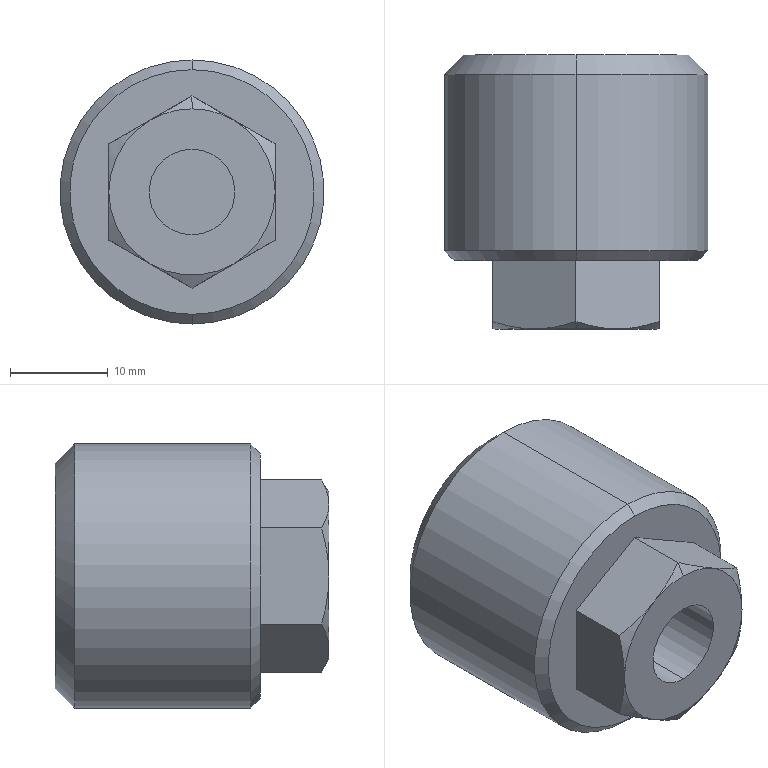Part | 1 solid | 29 faces | box 27 x 28 x 27 mm | volume 12379 mm3 | cone 11 | plane 10 | cylinder 6 | sphere 2 | commonest cylinder face diameters 8.75 x2 10 x2 27 x2
STEP:
#1=CARTESIAN_POINT('',(0.,18.,-5.));
#2=VERTEX_POINT('',#1);
#3=CARTESIAN_POINT('',(0.,18.,5.));
#4=VERTEX_POINT('',#3);
#5=CARTESIAN_POINT('',(0.,18.,0.));
#6=DIRECTION('',(0.,1.,0.));
#7=DIRECTION('',(0.,0.,-1.));
#8=AXIS2_PLACEMENT_3D('',#5,#6,#7);
#9=CIRCLE('',#8,5.);
#10=EDGE_CURVE('',#2,#4,#9,.T.);
#11=ORIENTED_EDGE('',*,*,#10,.T.);
#12=CARTESIAN_POINT('',(0.,13.,0.));
#13=VERTEX_POINT('',#12);
#14=CARTESIAN_POINT('',(0.,18.,0.));
#15=DIRECTION('',(1.,0.,0.));
#16=DIRECTION('',(0.,0.,-1.));
#17=AXIS2_PLACEMENT_3D('',#14,#15,#16);
#18=CIRCLE('',#17,5.);
#19=EDGE_CURVE('',#4,#13,#18,.T.);
#20=ORIENTED_EDGE('',*,*,#19,.T.);
#21=CARTESIAN_POINT('',(0.,18.,0.));
#22=DIRECTION('',(-1.,0.,0.));
#23=DIRECTION('',(0.,0.,1.));
#24=AXIS2_PLACEMENT_3D('',#21,#22,#23);
#25=CIRCLE('',#24,5.);
#26=EDGE_CURVE('',#2,#13,#25,.T.);
#27=ORIENTED_EDGE('',*,*,#26,.F.);
#28=EDGE_LOOP('',(#11,#20,#27));
#29=FACE_OUTER_BOUND('',#28,.T.);
#30=CARTESIAN_POINT('',(0.,18.,0.));
#31=DIRECTION('',(1.,0.,0.));
#32=DIRECTION('',(0.,0.,-1.));
#33=AXIS2_PLACEMENT_3D('',#30,#31,#32);
#34=SPHERICAL_SURFACE('',#33,5.);
#35=ADVANCED_FACE('',(#29),#34,.F.);
#36=CARTESIAN_POINT('',(0.,4.5,4.375));
#37=VERTEX_POINT('',#36);
#38=CARTESIAN_POINT('',(0.,4.5,-4.375));
#39=VERTEX_POINT('',#38);
#40=CARTESIAN_POINT('',(0.,4.5,0.));
#41=DIRECTION('',(0.,-1.,0.));
#42=DIRECTION('',(0.,0.,-1.));
#43=AXIS2_PLACEMENT_3D('',#40,#41,#42);
#44=CIRCLE('',#43,4.375);
#45=EDGE_CURVE('',#37,#39,#44,.T.);
#46=ORIENTED_EDGE('',*,*,#45,.F.);
#47=CARTESIAN_POINT('',(0.,-7.,4.375));
#48=VERTEX_POINT('',#47);
#49=CARTESIAN_POINT('',(0.,4.5,4.375));
#50=DIRECTION('',(0.,-1.,0.));
#51=VECTOR('',#50,1000.);
#52=LINE('',#49,#51);
#53=EDGE_CURVE('',#37,#48,#52,.T.);
#54=ORIENTED_EDGE('',*,*,#53,.T.);
#55=CARTESIAN_POINT('',(0.,-7.,-4.375));
#56=VERTEX_POINT('',#55);
#57=CARTESIAN_POINT('',(0.,-7.,0.));
#58=DIRECTION('',(0.,-1.,0.));
#59=DIRECTION('',(0.,0.,-1.));
#60=AXIS2_PLACEMENT_3D('',#57,#58,#59);
#61=CIRCLE('',#60,4.375);
#62=EDGE_CURVE('',#48,#56,#61,.T.);
#63=ORIENTED_EDGE('',*,*,#62,.T.);
#64=CARTESIAN_POINT('',(0.,4.5,-4.375));
#65=DIRECTION('',(0.,-1.,0.));
#66=VECTOR('',#65,1000.);
#67=LINE('',#64,#66);
#68=EDGE_CURVE('',#39,#56,#67,.T.);
#69=ORIENTED_EDGE('',*,*,#68,.F.);
#70=EDGE_LOOP('',(#46,#54,#63,#69));
#71=FACE_OUTER_BOUND('',#70,.T.);
#72=CARTESIAN_POINT('',(0.,4.5,0.));
#73=DIRECTION('',(0.,-1.,0.));
#74=DIRECTION('',(0.,0.,-1.));
#75=AXIS2_PLACEMENT_3D('',#72,#73,#74);
#76=CYLINDRICAL_SURFACE('',#75,4.375);
#77=ADVANCED_FACE('',(#71),#76,.F.);
#78=ORIENTED_EDGE('',*,*,#10,.F.);
#79=CARTESIAN_POINT('',(0.,21.,-5.));
#80=VERTEX_POINT('',#79);
#81=CARTESIAN_POINT('',(0.,18.,-5.));
#82=DIRECTION('',(0.,1.,0.));
#83=VECTOR('',#82,1000.);
#84=LINE('',#81,#83);
#85=EDGE_CURVE('',#2,#80,#84,.T.);
#86=ORIENTED_EDGE('',*,*,#85,.T.);
#87=CARTESIAN_POINT('',(0.,21.,5.));
#88=VERTEX_POINT('',#87);
#89=CARTESIAN_POINT('',(0.,21.,0.));
#90=DIRECTION('',(0.,-1.,0.));
#91=DIRECTION('',(0.,0.,-1.));
#92=AXIS2_PLACEMENT_3D('',#89,#90,#91);
#93=CIRCLE('',#92,5.);
#94=EDGE_CURVE('',#88,#80,#93,.T.);
#95=ORIENTED_EDGE('',*,*,#94,.F.);
#96=CARTESIAN_POINT('',(0.,18.,5.));
#97=DIRECTION('',(0.,1.,0.));
#98=VECTOR('',#97,1000.);
#99=LINE('',#96,#98);
#100=EDGE_CURVE('',#4,#88,#99,.T.);
#101=ORIENTED_EDGE('',*,*,#100,.F.);
#102=EDGE_LOOP('',(#78,#86,#95,#101));
#103=FACE_OUTER_BOUND('',#102,.T.);
#104=CARTESIAN_POINT('',(0.,18.,0.));
#105=DIRECTION('',(0.,1.,0.));
#106=DIRECTION('',(0.,0.,1.));
#107=AXIS2_PLACEMENT_3D('',#104,#105,#106);
#108=CYLINDRICAL_SURFACE('',#107,5.);
#109=ADVANCED_FACE('',(#103),#108,.F.);
#110=CARTESIAN_POINT('',(-4.25,-7.,7.361));
#111=VERTEX_POINT('',#110);
#112=CARTESIAN_POINT('',(0.,-7.,8.5));
#113=VERTEX_POINT('',#112);
#114=CARTESIAN_POINT('',(0.,-7.,0.));
#115=DIRECTION('',(0.,1.,0.));
#116=DIRECTION('',(0.,0.,1.));
#117=AXIS2_PLACEMENT_3D('',#114,#115,#116);
#118=CIRCLE('',#117,8.5);
#119=EDGE_CURVE('',#111,#113,#118,.T.);
#120=ORIENTED_EDGE('',*,*,#119,.T.);
#121=CARTESIAN_POINT('',(0.,-6.241,9.815));
#122=VERTEX_POINT('',#121);
#123=CARTESIAN_POINT('',(0.,8.034,34.54));
#124=DIRECTION('',(0.,0.5,0.866));
#125=VECTOR('',#124,1000.);
#126=LINE('',#123,#125);
#127=EDGE_CURVE('',#113,#122,#126,.T.);
#128=ORIENTED_EDGE('',*,*,#127,.T.);
#129=CARTESIAN_POINT('',(-4.25,-7.,7.361));
#130=CARTESIAN_POINT('',(-3.899,-7.,7.564));
#131=CARTESIAN_POINT('',(-3.367,-6.974,7.871));
#132=CARTESIAN_POINT('',(-2.737,-6.9,8.235));
#133=CARTESIAN_POINT('',(-2.42,-6.851,8.418));
#134=CARTESIAN_POINT('',(-2.26,-6.824,8.51));
#135=CARTESIAN_POINT('',(-2.18,-6.81,8.556));
#136=CARTESIAN_POINT('',(-2.146,-6.804,8.576));
#137=CARTESIAN_POINT('',(-2.123,-6.799,8.589));
#138=CARTESIAN_POINT('',(-2.111,-6.797,8.596));
#139=CARTESIAN_POINT('',(-1.437,-6.671,8.986));
#140=CARTESIAN_POINT('',(-0.7363,-6.486,9.39));
#141=CARTESIAN_POINT('',(0.,-6.241,9.815));
#142=B_SPLINE_CURVE_WITH_KNOTS('',3,(#129,#130,#131,#132,#133,#134,#135,#136,#137,#138,#139,#140,#141),.UNSPECIFIED.,.F.,.F.,(4,1,1,1,1,1,2,2,4),(0.,0.25,0.375,0.4375,0.4687,0.4844,0.4922,0.5,1.),.UNSPECIFIED.);
#143=EDGE_CURVE('',#111,#122,#142,.T.);
#144=ORIENTED_EDGE('',*,*,#143,.F.);
#145=EDGE_LOOP('',(#120,#128,#144));
#146=FACE_OUTER_BOUND('',#145,.T.);
#147=CARTESIAN_POINT('',(0.,8.034,0.));
#148=DIRECTION('',(0.,1.,0.));
#149=DIRECTION('',(0.,0.,1.));
#150=AXIS2_PLACEMENT_3D('',#147,#148,#149);
#151=CONICAL_SURFACE('',#150,34.54,1.047);
#152=ADVANCED_FACE('',(#146),#151,.T.);
#153=CARTESIAN_POINT('',(0.,0.,-12.5));
#154=VERTEX_POINT('',#153);
#155=CARTESIAN_POINT('',(0.,0.,12.5));
#156=VERTEX_POINT('',#155);
#157=CARTESIAN_POINT('',(0.,0.,0.));
#158=DIRECTION('',(0.,-1.,0.));
#159=DIRECTION('',(0.,0.,1.));
#160=AXIS2_PLACEMENT_3D('',#157,#158,#159);
#161=CIRCLE('',#160,12.5);
#162=EDGE_CURVE('',#154,#156,#161,.T.);
#163=ORIENTED_EDGE('',*,*,#162,.F.);
#164=CARTESIAN_POINT('',(0.,1.,-13.5));
#165=VERTEX_POINT('',#164);
#166=CARTESIAN_POINT('',(0.,1.,-13.5));
#167=DIRECTION('',(0.,0.7071,-0.7071));
#168=VECTOR('',#167,1000.);
#169=LINE('',#166,#168);
#170=EDGE_CURVE('',#154,#165,#169,.T.);
#171=ORIENTED_EDGE('',*,*,#170,.T.);
#172=CARTESIAN_POINT('',(0.,1.,13.5));
#173=VERTEX_POINT('',#172);
#174=CARTESIAN_POINT('',(0.,1.,0.));
#175=DIRECTION('',(0.,1.,0.));
#176=DIRECTION('',(0.,0.,1.));
#177=AXIS2_PLACEMENT_3D('',#174,#175,#176);
#178=CIRCLE('',#177,13.5);
#179=EDGE_CURVE('',#173,#165,#178,.T.);
#180=ORIENTED_EDGE('',*,*,#179,.F.);
#181=CARTESIAN_POINT('',(0.,1.,13.5));
#182=DIRECTION('',(0.,0.7071,0.7071));
#183=VECTOR('',#182,1000.);
#184=LINE('',#181,#183);
#185=EDGE_CURVE('',#156,#173,#184,.T.);
#186=ORIENTED_EDGE('',*,*,#185,.F.);
#187=EDGE_LOOP('',(#163,#171,#180,#186));
#188=FACE_OUTER_BOUND('',#187,.T.);
#189=CARTESIAN_POINT('',(0.,1.,0.));
#190=DIRECTION('',(0.,1.,0.));
#191=DIRECTION('',(0.,0.,1.));
#192=AXIS2_PLACEMENT_3D('',#189,#190,#191);
#193=CONICAL_SURFACE('',#192,13.5,0.7854);
#194=ADVANCED_FACE('',(#188),#193,.T.);
#195=CARTESIAN_POINT('',(0.,21.,11.5));
#196=VERTEX_POINT('',#195);
#197=CARTESIAN_POINT('',(0.,21.,-11.5));
#198=VERTEX_POINT('',#197);
#199=CARTESIAN_POINT('',(0.,21.,0.));
#200=DIRECTION('',(0.,1.,0.));
#201=DIRECTION('',(0.,0.,1.));
#202=AXIS2_PLACEMENT_3D('',#199,#200,#201);
#203=CIRCLE('',#202,11.5);
#204=EDGE_CURVE('',#196,#198,#203,.T.);
#205=ORIENTED_EDGE('',*,*,#204,.F.);
#206=CARTESIAN_POINT('',(0.,19.,13.5));
#207=VERTEX_POINT('',#206);
#208=CARTESIAN_POINT('',(0.,19.,13.5));
#209=DIRECTION('',(0.,-0.7071,0.7071));
#210=VECTOR('',#209,1000.);
#211=LINE('',#208,#210);
#212=EDGE_CURVE('',#196,#207,#211,.T.);
#213=ORIENTED_EDGE('',*,*,#212,.T.);
#214=CARTESIAN_POINT('',(0.,19.,-13.5));
#215=VERTEX_POINT('',#214);
#216=CARTESIAN_POINT('',(0.,19.,0.));
#217=DIRECTION('',(0.,1.,0.));
#218=DIRECTION('',(0.,0.,1.));
#219=AXIS2_PLACEMENT_3D('',#216,#217,#218);
#220=CIRCLE('',#219,13.5);
#221=EDGE_CURVE('',#207,#215,#220,.T.);
#222=ORIENTED_EDGE('',*,*,#221,.T.);
#223=CARTESIAN_POINT('',(0.,19.,-13.5));
#224=DIRECTION('',(0.,-0.7071,-0.7071));
#225=VECTOR('',#224,1000.);
#226=LINE('',#223,#225);
#227=EDGE_CURVE('',#198,#215,#226,.T.);
#228=ORIENTED_EDGE('',*,*,#227,.F.);
#229=EDGE_LOOP('',(#205,#213,#222,#228));
#230=FACE_OUTER_BOUND('',#229,.T.);
#231=CARTESIAN_POINT('',(0.,19.,0.));
#232=DIRECTION('',(0.,-1.,0.));
#233=DIRECTION('',(0.,0.,-1.));
#234=AXIS2_PLACEMENT_3D('',#231,#232,#233);
#235=CONICAL_SURFACE('',#234,13.5,0.7854);
#236=ADVANCED_FACE('',(#230),#235,.T.);
#237=ORIENTED_EDGE('',*,*,#179,.T.);
#238=CARTESIAN_POINT('',(0.,44.545,-13.5));
#239=DIRECTION('',(0.,1.,0.));
#240=VECTOR('',#239,1000.);
#241=LINE('',#238,#240);
#242=EDGE_CURVE('',#165,#215,#241,.T.);
#243=ORIENTED_EDGE('',*,*,#242,.T.);
#244=ORIENTED_EDGE('',*,*,#221,.F.);
#245=CARTESIAN_POINT('',(0.,44.545,13.5));
#246=DIRECTION('',(0.,1.,0.));
#247=VECTOR('',#246,1000.);
#248=LINE('',#245,#247);
#249=EDGE_CURVE('',#173,#207,#248,.T.);
#250=ORIENTED_EDGE('',*,*,#249,.F.);
#251=EDGE_LOOP('',(#237,#243,#244,#250));
#252=FACE_OUTER_BOUND('',#251,.T.);
#253=CARTESIAN_POINT('',(0.,44.545,0.));
#254=DIRECTION('',(0.,1.,0.));
#255=DIRECTION('',(0.,0.,1.));
#256=AXIS2_PLACEMENT_3D('',#253,#254,#255);
#257=CYLINDRICAL_SURFACE('',#256,13.5);
#258=ADVANCED_FACE('',(#252),#257,.T.);
#259=CARTESIAN_POINT('',(0.,0.,9.815));
#260=VERTEX_POINT('',#259);
#261=CARTESIAN_POINT('',(0.,-7.,9.815));
#262=DIRECTION('',(0.,1.,0.));
#263=VECTOR('',#262,1000.);
#264=LINE('',#261,#263);
#265=EDGE_CURVE('',#122,#260,#264,.T.);
#266=ORIENTED_EDGE('',*,*,#265,.F.);
#267=CARTESIAN_POINT('',(4.25,-7.,7.361));
#268=VERTEX_POINT('',#267);
#269=CARTESIAN_POINT('',(0.,-6.241,9.815));
#270=CARTESIAN_POINT('',(0.3685,-6.364,9.602));
#271=CARTESIAN_POINT('',(0.9078,-6.525,9.291));
#272=CARTESIAN_POINT('',(1.513,-6.674,8.941));
#273=CARTESIAN_POINT('',(1.81,-6.738,8.77));
#274=CARTESIAN_POINT('',(1.957,-6.768,8.685));
#275=CARTESIAN_POINT('',(2.03,-6.782,8.643));
#276=CARTESIAN_POINT('',(2.062,-6.788,8.625));
#277=CARTESIAN_POINT('',(2.082,-6.792,8.613));
#278=CARTESIAN_POINT('',(2.092,-6.793,8.607));
#279=CARTESIAN_POINT('',(2.833,-6.932,8.179));
#280=CARTESIAN_POINT('',(3.549,-7.,7.766));
#281=CARTESIAN_POINT('',(4.25,-7.,7.361));
#282=B_SPLINE_CURVE_WITH_KNOTS('',3,(#269,#270,#271,#272,#273,#274,#275,#276,#277,#278,#279,#280,#281),.UNSPECIFIED.,.F.,.F.,(4,1,1,1,1,1,2,2,4),(0.,0.25,0.375,0.4375,0.4687,0.4844,0.4922,0.5,1.),.UNSPECIFIED.);
#283=EDGE_CURVE('',#122,#268,#282,.T.);
#284=ORIENTED_EDGE('',*,*,#283,.T.);
#285=CARTESIAN_POINT('',(8.5,-6.241,4.907));
#286=VERTEX_POINT('',#285);
#287=CARTESIAN_POINT('',(4.25,-7.,7.361));
#288=CARTESIAN_POINT('',(4.601,-7.,7.159));
#289=CARTESIAN_POINT('',(5.133,-6.974,6.852));
#290=CARTESIAN_POINT('',(5.763,-6.9,6.488));
#291=CARTESIAN_POINT('',(6.08,-6.851,6.304));
#292=CARTESIAN_POINT('',(6.24,-6.824,6.212));
#293=CARTESIAN_POINT('',(6.32,-6.81,6.166));
#294=CARTESIAN_POINT('',(6.354,-6.804,6.147));
#295=CARTESIAN_POINT('',(6.377,-6.799,6.133));
#296=CARTESIAN_POINT('',(6.389,-6.797,6.126));
#297=CARTESIAN_POINT('',(7.063,-6.671,5.737));
#298=CARTESIAN_POINT('',(7.764,-6.486,5.333));
#299=CARTESIAN_POINT('',(8.5,-6.241,4.907));
#300=B_SPLINE_CURVE_WITH_KNOTS('',3,(#287,#288,#289,#290,#291,#292,#293,#294,#295,#296,#297,#298,#299),.UNSPECIFIED.,.F.,.F.,(4,1,1,1,1,1,2,2,4),(0.,0.25,0.375,0.4375,0.4688,0.4844,0.4922,0.5,1.),.UNSPECIFIED.);
#301=EDGE_CURVE('',#268,#286,#300,.T.);
#302=ORIENTED_EDGE('',*,*,#301,.T.);
#303=CARTESIAN_POINT('',(8.5,0.,4.907));
#304=VERTEX_POINT('',#303);
#305=CARTESIAN_POINT('',(8.5,-7.,4.907));
#306=DIRECTION('',(0.,1.,0.));
#307=VECTOR('',#306,1000.);
#308=LINE('',#305,#307);
#309=EDGE_CURVE('',#286,#304,#308,.T.);
#310=ORIENTED_EDGE('',*,*,#309,.T.);
#311=CARTESIAN_POINT('',(0.,0.,9.815));
#312=DIRECTION('',(0.866,0.,-0.5));
#313=VECTOR('',#312,1000.);
#314=LINE('',#311,#313);
#315=EDGE_CURVE('',#260,#304,#314,.T.);
#316=ORIENTED_EDGE('',*,*,#315,.F.);
#317=EDGE_LOOP('',(#266,#284,#302,#310,#316));
#318=FACE_OUTER_BOUND('',#317,.T.);
#319=CARTESIAN_POINT('',(0.,-7.,9.815));
#320=DIRECTION('',(0.5,0.,0.866));
#321=DIRECTION('',(0.,-1.,0.));
#322=AXIS2_PLACEMENT_3D('',#319,#320,#321);
#323=PLANE('',#322);
#324=ADVANCED_FACE('',(#318),#323,.T.);
#325=CARTESIAN_POINT('',(-8.5,-6.241,4.907));
#326=VERTEX_POINT('',#325);
#327=CARTESIAN_POINT('',(-8.5,0.,4.907));
#328=VERTEX_POINT('',#327);
#329=CARTESIAN_POINT('',(-8.5,-7.,4.907));
#330=DIRECTION('',(0.,1.,0.));
#331=VECTOR('',#330,1000.);
#332=LINE('',#329,#331);
#333=EDGE_CURVE('',#326,#328,#332,.T.);
#334=ORIENTED_EDGE('',*,*,#333,.F.);
#335=CARTESIAN_POINT('',(-8.5,-6.241,4.907));
#336=CARTESIAN_POINT('',(-8.132,-6.364,5.12));
#337=CARTESIAN_POINT('',(-7.592,-6.525,5.432));
#338=CARTESIAN_POINT('',(-6.987,-6.674,5.781));
#339=CARTESIAN_POINT('',(-6.69,-6.738,5.953));
#340=CARTESIAN_POINT('',(-6.543,-6.768,6.037));
#341=CARTESIAN_POINT('',(-6.47,-6.782,6.08));
#342=CARTESIAN_POINT('',(-6.438,-6.788,6.098));
#343=CARTESIAN_POINT('',(-6.418,-6.792,6.11));
#344=CARTESIAN_POINT('',(-6.408,-6.793,6.115));
#345=CARTESIAN_POINT('',(-5.667,-6.932,6.543));
#346=CARTESIAN_POINT('',(-4.951,-7.,6.956));
#347=CARTESIAN_POINT('',(-4.25,-7.,7.361));
#348=B_SPLINE_CURVE_WITH_KNOTS('',3,(#335,#336,#337,#338,#339,#340,#341,#342,#343,#344,#345,#346,#347),.UNSPECIFIED.,.F.,.F.,(4,1,1,1,1,1,2,2,4),(0.,0.25,0.375,0.4375,0.4687,0.4844,0.4922,0.5,1.),.UNSPECIFIED.);
#349=EDGE_CURVE('',#326,#111,#348,.T.);
#350=ORIENTED_EDGE('',*,*,#349,.T.);
#351=ORIENTED_EDGE('',*,*,#143,.T.);
#352=ORIENTED_EDGE('',*,*,#265,.T.);
#353=CARTESIAN_POINT('',(-8.5,0.,4.907));
#354=DIRECTION('',(0.866,0.,0.5));
#355=VECTOR('',#354,1000.);
#356=LINE('',#353,#355);
#357=EDGE_CURVE('',#328,#260,#356,.T.);
#358=ORIENTED_EDGE('',*,*,#357,.F.);
#359=EDGE_LOOP('',(#334,#350,#351,#352,#358));
#360=FACE_OUTER_BOUND('',#359,.T.);
#361=CARTESIAN_POINT('',(-8.5,-7.,4.907));
#362=DIRECTION('',(-0.5,0.,0.866));
#363=DIRECTION('',(0.,1.,0.));
#364=AXIS2_PLACEMENT_3D('',#361,#362,#363);
#365=PLANE('',#364);
#366=ADVANCED_FACE('',(#360),#365,.T.);
#367=CARTESIAN_POINT('',(-8.5,-6.241,-4.907));
#368=VERTEX_POINT('',#367);
#369=CARTESIAN_POINT('',(-8.5,0.,-4.907));
#370=VERTEX_POINT('',#369);
#371=CARTESIAN_POINT('',(-8.5,-7.,-4.907));
#372=DIRECTION('',(0.,1.,0.));
#373=VECTOR('',#372,1000.);
#374=LINE('',#371,#373);
#375=EDGE_CURVE('',#368,#370,#374,.T.);
#376=ORIENTED_EDGE('',*,*,#375,.F.);
#377=CARTESIAN_POINT('',(-8.5,-7.,0.));
#378=VERTEX_POINT('',#377);
#379=CARTESIAN_POINT('',(-8.5,-6.241,-4.907));
#380=CARTESIAN_POINT('',(-8.5,-6.364,-4.481));
#381=CARTESIAN_POINT('',(-8.5,-6.526,-3.857));
#382=CARTESIAN_POINT('',(-8.5,-6.674,-3.156));
#383=CARTESIAN_POINT('',(-8.5,-6.739,-2.812));
#384=CARTESIAN_POINT('',(-8.5,-6.769,-2.642));
#385=CARTESIAN_POINT('',(-8.5,-6.781,-2.569));
#386=CARTESIAN_POINT('',(-8.5,-6.789,-2.521));
#387=CARTESIAN_POINT('',(-8.5,-6.792,-2.499));
#388=CARTESIAN_POINT('',(-8.5,-6.932,-1.632));
#389=CARTESIAN_POINT('',(-8.5,-7.,-0.8078));
#390=CARTESIAN_POINT('',(-8.5,-7.,0.));
#391=B_SPLINE_CURVE_WITH_KNOTS('',3,(#379,#380,#381,#382,#383,#384,#385,#386,#387,#388,#389,#390),.UNSPECIFIED.,.F.,.F.,(4,1,1,1,1,2,2,4),(0.,0.25,0.375,0.4375,0.4688,0.4844,0.5,1.),.UNSPECIFIED.);
#392=EDGE_CURVE('',#368,#378,#391,.T.);
#393=ORIENTED_EDGE('',*,*,#392,.T.);
#394=CARTESIAN_POINT('',(-8.5,-7.,0.));
#395=CARTESIAN_POINT('',(-8.5,-7.,0.4066));
#396=CARTESIAN_POINT('',(-8.5,-6.974,1.023));
#397=CARTESIAN_POINT('',(-8.5,-6.899,1.753));
#398=CARTESIAN_POINT('',(-8.5,-6.85,2.121));
#399=CARTESIAN_POINT('',(-8.5,-6.823,2.306));
#400=CARTESIAN_POINT('',(-8.5,-6.808,2.399));
#401=CARTESIAN_POINT('',(-8.5,-6.802,2.438));
#402=CARTESIAN_POINT('',(-8.5,-6.798,2.465));
#403=CARTESIAN_POINT('',(-8.5,-6.796,2.479));
#404=CARTESIAN_POINT('',(-8.5,-6.67,3.255));
#405=CARTESIAN_POINT('',(-8.5,-6.485,4.061));
#406=CARTESIAN_POINT('',(-8.5,-6.241,4.907));
#407=B_SPLINE_CURVE_WITH_KNOTS('',3,(#394,#395,#396,#397,#398,#399,#400,#401,#402,#403,#404,#405,#406),.UNSPECIFIED.,.F.,.F.,(4,1,1,1,1,1,2,2,4),(0.,0.25,0.375,0.4375,0.4688,0.4844,0.4922,0.5,1.),.UNSPECIFIED.);
#408=EDGE_CURVE('',#378,#326,#407,.T.);
#409=ORIENTED_EDGE('',*,*,#408,.T.);
#410=ORIENTED_EDGE('',*,*,#333,.T.);
#411=CARTESIAN_POINT('',(-8.5,0.,-4.907));
#412=DIRECTION('',(0.,0.,1.));
#413=VECTOR('',#412,1000.);
#414=LINE('',#411,#413);
#415=EDGE_CURVE('',#370,#328,#414,.T.);
#416=ORIENTED_EDGE('',*,*,#415,.F.);
#417=EDGE_LOOP('',(#376,#393,#409,#410,#416));
#418=FACE_OUTER_BOUND('',#417,.T.);
#419=CARTESIAN_POINT('',(-8.5,-7.,-4.907));
#420=DIRECTION('',(-1.,0.,0.));
#421=DIRECTION('',(0.,1.,0.));
#422=AXIS2_PLACEMENT_3D('',#419,#420,#421);
#423=PLANE('',#422);
#424=ADVANCED_FACE('',(#418),#423,.T.);
#425=CARTESIAN_POINT('',(0.,-6.241,-9.815));
#426=VERTEX_POINT('',#425);
#427=CARTESIAN_POINT('',(0.,0.,-9.815));
#428=VERTEX_POINT('',#427);
#429=CARTESIAN_POINT('',(0.,-7.,-9.815));
#430=DIRECTION('',(0.,1.,0.));
#431=VECTOR('',#430,1000.);
#432=LINE('',#429,#431);
#433=EDGE_CURVE('',#426,#428,#432,.T.);
#434=ORIENTED_EDGE('',*,*,#433,.F.);
#435=CARTESIAN_POINT('',(-4.25,-7.,-7.361));
#436=VERTEX_POINT('',#435);
#437=CARTESIAN_POINT('',(0.,-6.241,-9.815));
#438=CARTESIAN_POINT('',(-0.3685,-6.364,-9.602));
#439=CARTESIAN_POINT('',(-0.9078,-6.525,-9.291));
#440=CARTESIAN_POINT('',(-1.513,-6.674,-8.941));
#441=CARTESIAN_POINT('',(-1.81,-6.738,-8.77));
#442=CARTESIAN_POINT('',(-1.957,-6.768,-8.685));
#443=CARTESIAN_POINT('',(-2.03,-6.782,-8.643));
#444=CARTESIAN_POINT('',(-2.062,-6.788,-8.625));
#445=CARTESIAN_POINT('',(-2.082,-6.792,-8.613));
#446=CARTESIAN_POINT('',(-2.092,-6.793,-8.607));
#447=CARTESIAN_POINT('',(-2.833,-6.932,-8.179));
#448=CARTESIAN_POINT('',(-3.549,-7.,-7.766));
#449=CARTESIAN_POINT('',(-4.25,-7.,-7.361));
#450=B_SPLINE_CURVE_WITH_KNOTS('',3,(#437,#438,#439,#440,#441,#442,#443,#444,#445,#446,#447,#448,#449),.UNSPECIFIED.,.F.,.F.,(4,1,1,1,1,1,2,2,4),(0.,0.25,0.375,0.4375,0.4688,0.4844,0.4922,0.5,1.),.UNSPECIFIED.);
#451=EDGE_CURVE('',#426,#436,#450,.T.);
#452=ORIENTED_EDGE('',*,*,#451,.T.);
#453=CARTESIAN_POINT('',(-4.25,-7.,-7.361));
#454=CARTESIAN_POINT('',(-4.601,-7.,-7.159));
#455=CARTESIAN_POINT('',(-5.133,-6.974,-6.852));
#456=CARTESIAN_POINT('',(-5.763,-6.9,-6.488));
#457=CARTESIAN_POINT('',(-6.08,-6.851,-6.304));
#458=CARTESIAN_POINT('',(-6.24,-6.824,-6.212));
#459=CARTESIAN_POINT('',(-6.32,-6.81,-6.166));
#460=CARTESIAN_POINT('',(-6.354,-6.804,-6.147));
#461=CARTESIAN_POINT('',(-6.377,-6.799,-6.133));
#462=CARTESIAN_POINT('',(-6.389,-6.797,-6.126));
#463=CARTESIAN_POINT('',(-7.063,-6.671,-5.737));
#464=CARTESIAN_POINT('',(-7.764,-6.486,-5.333));
#465=CARTESIAN_POINT('',(-8.5,-6.241,-4.907));
#466=B_SPLINE_CURVE_WITH_KNOTS('',3,(#453,#454,#455,#456,#457,#458,#459,#460,#461,#462,#463,#464,#465),.UNSPECIFIED.,.F.,.F.,(4,1,1,1,1,1,2,2,4),(0.,0.25,0.375,0.4375,0.4687,0.4844,0.4922,0.5,1.),.UNSPECIFIED.);
#467=EDGE_CURVE('',#436,#368,#466,.T.);
#468=ORIENTED_EDGE('',*,*,#467,.T.);
#469=ORIENTED_EDGE('',*,*,#375,.T.);
#470=CARTESIAN_POINT('',(0.,0.,-9.815));
#471=DIRECTION('',(-0.866,0.,0.5));
#472=VECTOR('',#471,1000.);
#473=LINE('',#470,#472);
#474=EDGE_CURVE('',#428,#370,#473,.T.);
#475=ORIENTED_EDGE('',*,*,#474,.F.);
#476=EDGE_LOOP('',(#434,#452,#468,#469,#475));
#477=FACE_OUTER_BOUND('',#476,.T.);
#478=CARTESIAN_POINT('',(0.,-7.,-9.815));
#479=DIRECTION('',(-0.5,0.,-0.866));
#480=DIRECTION('',(-0.866,0.,0.5));
#481=AXIS2_PLACEMENT_3D('',#478,#479,#480);
#482=PLANE('',#481);
#483=ADVANCED_FACE('',(#477),#482,.T.);
#484=CARTESIAN_POINT('',(8.5,-6.241,-4.907));
#485=VERTEX_POINT('',#484);
#486=CARTESIAN_POINT('',(8.5,0.,-4.907));
#487=VERTEX_POINT('',#486);
#488=CARTESIAN_POINT('',(8.5,-7.,-4.907));
#489=DIRECTION('',(0.,1.,0.));
#490=VECTOR('',#489,1000.);
#491=LINE('',#488,#490);
#492=EDGE_CURVE('',#485,#487,#491,.T.);
#493=ORIENTED_EDGE('',*,*,#492,.F.);
#494=CARTESIAN_POINT('',(4.25,-7.,-7.361));
#495=VERTEX_POINT('',#494);
#496=CARTESIAN_POINT('',(8.5,-6.241,-4.907));
#497=CARTESIAN_POINT('',(8.132,-6.364,-5.12));
#498=CARTESIAN_POINT('',(7.592,-6.525,-5.432));
#499=CARTESIAN_POINT('',(6.987,-6.674,-5.781));
#500=CARTESIAN_POINT('',(6.69,-6.738,-5.953));
#501=CARTESIAN_POINT('',(6.543,-6.768,-6.037));
#502=CARTESIAN_POINT('',(6.47,-6.782,-6.08));
#503=CARTESIAN_POINT('',(6.438,-6.788,-6.098));
#504=CARTESIAN_POINT('',(6.418,-6.792,-6.11));
#505=CARTESIAN_POINT('',(6.408,-6.793,-6.115));
#506=CARTESIAN_POINT('',(5.667,-6.932,-6.543));
#507=CARTESIAN_POINT('',(4.951,-7.,-6.956));
#508=CARTESIAN_POINT('',(4.25,-7.,-7.361));
#509=B_SPLINE_CURVE_WITH_KNOTS('',3,(#496,#497,#498,#499,#500,#501,#502,#503,#504,#505,#506,#507,#508),.UNSPECIFIED.,.F.,.F.,(4,1,1,1,1,1,2,2,4),(0.,0.25,0.375,0.4375,0.4687,0.4844,0.4922,0.5,1.),.UNSPECIFIED.);
#510=EDGE_CURVE('',#485,#495,#509,.T.);
#511=ORIENTED_EDGE('',*,*,#510,.T.);
#512=CARTESIAN_POINT('',(4.25,-7.,-7.361));
#513=CARTESIAN_POINT('',(3.899,-7.,-7.564));
#514=CARTESIAN_POINT('',(3.367,-6.974,-7.871));
#515=CARTESIAN_POINT('',(2.737,-6.9,-8.235));
#516=CARTESIAN_POINT('',(2.42,-6.851,-8.418));
#517=CARTESIAN_POINT('',(2.26,-6.824,-8.51));
#518=CARTESIAN_POINT('',(2.18,-6.81,-8.556));
#519=CARTESIAN_POINT('',(2.146,-6.804,-8.576));
#520=CARTESIAN_POINT('',(2.123,-6.799,-8.589));
#521=CARTESIAN_POINT('',(2.111,-6.797,-8.596));
#522=CARTESIAN_POINT('',(1.437,-6.671,-8.986));
#523=CARTESIAN_POINT('',(0.7363,-6.486,-9.39));
#524=CARTESIAN_POINT('',(0.,-6.241,-9.815));
#525=B_SPLINE_CURVE_WITH_KNOTS('',3,(#512,#513,#514,#515,#516,#517,#518,#519,#520,#521,#522,#523,#524),.UNSPECIFIED.,.F.,.F.,(4,1,1,1,1,1,2,2,4),(0.,0.25,0.375,0.4375,0.4687,0.4844,0.4922,0.5,1.),.UNSPECIFIED.);
#526=EDGE_CURVE('',#495,#426,#525,.T.);
#527=ORIENTED_EDGE('',*,*,#526,.T.);
#528=ORIENTED_EDGE('',*,*,#433,.T.);
#529=CARTESIAN_POINT('',(8.5,0.,-4.907));
#530=DIRECTION('',(-0.866,0.,-0.5));
#531=VECTOR('',#530,1000.);
#532=LINE('',#529,#531);
#533=EDGE_CURVE('',#487,#428,#532,.T.);
#534=ORIENTED_EDGE('',*,*,#533,.F.);
#535=EDGE_LOOP('',(#493,#511,#527,#528,#534));
#536=FACE_OUTER_BOUND('',#535,.T.);
#537=CARTESIAN_POINT('',(8.5,-7.,-4.907));
#538=DIRECTION('',(0.5,0.,-0.866));
#539=DIRECTION('',(0.,-1.,0.));
#540=AXIS2_PLACEMENT_3D('',#537,#538,#539);
#541=PLANE('',#540);
#542=ADVANCED_FACE('',(#536),#541,.T.);
#543=ORIENTED_EDGE('',*,*,#309,.F.);
#544=CARTESIAN_POINT('',(8.5,-7.,0.));
#545=VERTEX_POINT('',#544);
#546=CARTESIAN_POINT('',(8.5,-6.241,4.907));
#547=CARTESIAN_POINT('',(8.5,-6.363,4.484));
#548=CARTESIAN_POINT('',(8.5,-6.524,3.865));
#549=CARTESIAN_POINT('',(8.5,-6.672,3.169));
#550=CARTESIAN_POINT('',(8.5,-6.736,2.828));
#551=CARTESIAN_POINT('',(8.5,-6.766,2.659));
#552=CARTESIAN_POINT('',(8.5,-6.78,2.575));
#553=CARTESIAN_POINT('',(8.5,-6.786,2.539));
#554=CARTESIAN_POINT('',(8.5,-6.79,2.515));
#555=CARTESIAN_POINT('',(8.5,-6.791,2.504));
#556=CARTESIAN_POINT('',(8.5,-6.931,1.644));
#557=CARTESIAN_POINT('',(8.5,-7.,0.8135));
#558=CARTESIAN_POINT('',(8.5,-7.,0.));
#559=B_SPLINE_CURVE_WITH_KNOTS('',3,(#546,#547,#548,#549,#550,#551,#552,#553,#554,#555,#556,#557,#558),.UNSPECIFIED.,.F.,.F.,(4,1,1,1,1,1,2,2,4),(0.,0.25,0.375,0.4375,0.4687,0.4844,0.4922,0.5,1.),.UNSPECIFIED.);
#560=EDGE_CURVE('',#286,#545,#559,.T.);
#561=ORIENTED_EDGE('',*,*,#560,.T.);
#562=CARTESIAN_POINT('',(8.5,-7.,0.));
#563=CARTESIAN_POINT('',(8.5,-7.,-0.4037));
#564=CARTESIAN_POINT('',(8.5,-6.975,-1.016));
#565=CARTESIAN_POINT('',(8.5,-6.9,-1.741));
#566=CARTESIAN_POINT('',(8.5,-6.852,-2.106));
#567=CARTESIAN_POINT('',(8.5,-6.825,-2.289));
#568=CARTESIAN_POINT('',(8.5,-6.811,-2.381));
#569=CARTESIAN_POINT('',(8.5,-6.805,-2.42));
#570=CARTESIAN_POINT('',(8.5,-6.801,-2.447));
#571=CARTESIAN_POINT('',(8.5,-6.798,-2.461));
#572=CARTESIAN_POINT('',(8.5,-6.672,-3.242));
#573=CARTESIAN_POINT('',(8.5,-6.487,-4.054));
#574=CARTESIAN_POINT('',(8.5,-6.241,-4.907));
#575=B_SPLINE_CURVE_WITH_KNOTS('',3,(#562,#563,#564,#565,#566,#567,#568,#569,#570,#571,#572,#573,#574),.UNSPECIFIED.,.F.,.F.,(4,1,1,1,1,1,2,2,4),(0.,0.25,0.375,0.4375,0.4688,0.4844,0.4922,0.5,1.),.UNSPECIFIED.);
#576=EDGE_CURVE('',#545,#485,#575,.T.);
#577=ORIENTED_EDGE('',*,*,#576,.T.);
#578=ORIENTED_EDGE('',*,*,#492,.T.);
#579=CARTESIAN_POINT('',(8.5,0.,4.907));
#580=DIRECTION('',(0.,0.,-1.));
#581=VECTOR('',#580,1000.);
#582=LINE('',#579,#581);
#583=EDGE_CURVE('',#304,#487,#582,.T.);
#584=ORIENTED_EDGE('',*,*,#583,.F.);
#585=EDGE_LOOP('',(#543,#561,#577,#578,#584));
#586=FACE_OUTER_BOUND('',#585,.T.);
#587=CARTESIAN_POINT('',(8.5,-7.,4.907));
#588=DIRECTION('',(1.,0.,0.));
#589=DIRECTION('',(0.,1.,0.));
#590=AXIS2_PLACEMENT_3D('',#587,#588,#589);
#591=PLANE('',#590);
#592=ADVANCED_FACE('',(#586),#591,.T.);
#593=CARTESIAN_POINT('',(0.,0.,0.));
#594=DIRECTION('',(0.,-1.,0.));
#595=DIRECTION('',(0.,0.,1.));
#596=AXIS2_PLACEMENT_3D('',#593,#594,#595);
#597=CIRCLE('',#596,12.5);
#598=EDGE_CURVE('',#156,#154,#597,.T.);
#599=ORIENTED_EDGE('',*,*,#598,.T.);
#600=ORIENTED_EDGE('',*,*,#162,.T.);
#601=EDGE_LOOP('',(#599,#600));
#602=FACE_OUTER_BOUND('',#601,.T.);
#603=ORIENTED_EDGE('',*,*,#357,.T.);
#604=ORIENTED_EDGE('',*,*,#315,.T.);
#605=ORIENTED_EDGE('',*,*,#583,.T.);
#606=ORIENTED_EDGE('',*,*,#533,.T.);
#607=ORIENTED_EDGE('',*,*,#474,.T.);
#608=ORIENTED_EDGE('',*,*,#415,.T.);
#609=EDGE_LOOP('',(#603,#604,#605,#606,#607,#608));
#610=FACE_BOUND('',#609,.T.);
#611=CARTESIAN_POINT('',(0.,0.,0.));
#612=DIRECTION('',(0.,1.,0.));
#613=DIRECTION('',(1.,0.,0.));
#614=AXIS2_PLACEMENT_3D('',#611,#612,#613);
#615=PLANE('',#614);
#616=ADVANCED_FACE('',(#602,#610),#615,.F.);
#617=ORIENTED_EDGE('',*,*,#242,.F.);
#618=CARTESIAN_POINT('',(0.,1.,0.));
#619=DIRECTION('',(0.,1.,0.));
#620=DIRECTION('',(0.,0.,1.));
#621=AXIS2_PLACEMENT_3D('',#618,#619,#620);
#622=CIRCLE('',#621,13.5);
#623=EDGE_CURVE('',#165,#173,#622,.T.);
#624=ORIENTED_EDGE('',*,*,#623,.T.);
#625=ORIENTED_EDGE('',*,*,#249,.T.);
#626=CARTESIAN_POINT('',(0.,19.,0.));
#627=DIRECTION('',(0.,1.,0.));
#628=DIRECTION('',(0.,0.,1.));
#629=AXIS2_PLACEMENT_3D('',#626,#627,#628);
#630=CIRCLE('',#629,13.5);
#631=EDGE_CURVE('',#215,#207,#630,.T.);
#632=ORIENTED_EDGE('',*,*,#631,.F.);
#633=EDGE_LOOP('',(#617,#624,#625,#632));
#634=FACE_OUTER_BOUND('',#633,.T.);
#635=CARTESIAN_POINT('',(0.,44.545,0.));
#636=DIRECTION('',(0.,1.,0.));
#637=DIRECTION('',(0.,0.,1.));
#638=AXIS2_PLACEMENT_3D('',#635,#636,#637);
#639=CYLINDRICAL_SURFACE('',#638,13.5);
#640=ADVANCED_FACE('',(#634),#639,.T.);
#641=ORIENTED_EDGE('',*,*,#212,.F.);
#642=CARTESIAN_POINT('',(0.,21.,0.));
#643=DIRECTION('',(0.,1.,0.));
#644=DIRECTION('',(0.,0.,1.));
#645=AXIS2_PLACEMENT_3D('',#642,#643,#644);
#646=CIRCLE('',#645,11.5);
#647=EDGE_CURVE('',#198,#196,#646,.T.);
#648=ORIENTED_EDGE('',*,*,#647,.F.);
#649=ORIENTED_EDGE('',*,*,#227,.T.);
#650=ORIENTED_EDGE('',*,*,#631,.T.);
#651=EDGE_LOOP('',(#641,#648,#649,#650));
#652=FACE_OUTER_BOUND('',#651,.T.);
#653=CARTESIAN_POINT('',(0.,19.,0.));
#654=DIRECTION('',(0.,-1.,0.));
#655=DIRECTION('',(0.,0.,-1.));
#656=AXIS2_PLACEMENT_3D('',#653,#654,#655);
#657=CONICAL_SURFACE('',#656,13.5,0.7854);
#658=ADVANCED_FACE('',(#652),#657,.T.);
#659=ORIENTED_EDGE('',*,*,#647,.T.);
#660=ORIENTED_EDGE('',*,*,#204,.T.);
#661=EDGE_LOOP('',(#659,#660));
#662=FACE_OUTER_BOUND('',#661,.T.);
#663=ORIENTED_EDGE('',*,*,#94,.T.);
#664=CARTESIAN_POINT('',(0.,21.,0.));
#665=DIRECTION('',(0.,-1.,0.));
#666=DIRECTION('',(0.,0.,-1.));
#667=AXIS2_PLACEMENT_3D('',#664,#665,#666);
#668=CIRCLE('',#667,5.);
#669=EDGE_CURVE('',#80,#88,#668,.T.);
#670=ORIENTED_EDGE('',*,*,#669,.T.);
#671=EDGE_LOOP('',(#663,#670));
#672=FACE_BOUND('',#671,.T.);
#673=CARTESIAN_POINT('',(11.5,21.,0.));
#674=DIRECTION('',(0.,-1.,0.));
#675=DIRECTION('',(0.,0.,-1.));
#676=AXIS2_PLACEMENT_3D('',#673,#674,#675);
#677=PLANE('',#676);
#678=ADVANCED_FACE('',(#662,#672),#677,.F.);
#679=ORIENTED_EDGE('',*,*,#170,.F.);
#680=ORIENTED_EDGE('',*,*,#598,.F.);
#681=ORIENTED_EDGE('',*,*,#185,.T.);
#682=ORIENTED_EDGE('',*,*,#623,.F.);
#683=EDGE_LOOP('',(#679,#680,#681,#682));
#684=FACE_OUTER_BOUND('',#683,.T.);
#685=CARTESIAN_POINT('',(0.,1.,0.));
#686=DIRECTION('',(0.,1.,0.));
#687=DIRECTION('',(0.,0.,1.));
#688=AXIS2_PLACEMENT_3D('',#685,#686,#687);
#689=CONICAL_SURFACE('',#688,13.5,0.7854);
#690=ADVANCED_FACE('',(#684),#689,.T.);
#691=ORIENTED_EDGE('',*,*,#127,.F.);
#692=CARTESIAN_POINT('',(0.,-7.,0.));
#693=DIRECTION('',(0.,1.,0.));
#694=DIRECTION('',(0.,0.,1.));
#695=AXIS2_PLACEMENT_3D('',#692,#693,#694);
#696=CIRCLE('',#695,8.5);
#697=EDGE_CURVE('',#113,#268,#696,.T.);
#698=ORIENTED_EDGE('',*,*,#697,.T.);
#699=ORIENTED_EDGE('',*,*,#283,.F.);
#700=EDGE_LOOP('',(#691,#698,#699));
#701=FACE_OUTER_BOUND('',#700,.T.);
#702=CARTESIAN_POINT('',(0.,8.034,0.));
#703=DIRECTION('',(0.,1.,0.));
#704=DIRECTION('',(0.,0.,1.));
#705=AXIS2_PLACEMENT_3D('',#702,#703,#704);
#706=CONICAL_SURFACE('',#705,34.54,1.047);
#707=ADVANCED_FACE('',(#701),#706,.T.);
#708=CARTESIAN_POINT('',(0.,-7.,0.));
#709=DIRECTION('',(0.,1.,0.));
#710=DIRECTION('',(0.,0.,1.));
#711=AXIS2_PLACEMENT_3D('',#708,#709,#710);
#712=CIRCLE('',#711,8.5);
#713=EDGE_CURVE('',#378,#111,#712,.T.);
#714=ORIENTED_EDGE('',*,*,#713,.T.);
#715=ORIENTED_EDGE('',*,*,#349,.F.);
#716=ORIENTED_EDGE('',*,*,#408,.F.);
#717=EDGE_LOOP('',(#714,#715,#716));
#718=FACE_OUTER_BOUND('',#717,.T.);
#719=CARTESIAN_POINT('',(0.,8.034,0.));
#720=DIRECTION('',(0.,1.,0.));
#721=DIRECTION('',(0.,0.,1.));
#722=AXIS2_PLACEMENT_3D('',#719,#720,#721);
#723=CONICAL_SURFACE('',#722,34.54,1.047);
#724=ADVANCED_FACE('',(#718),#723,.T.);
#725=ORIENTED_EDGE('',*,*,#467,.F.);
#726=CARTESIAN_POINT('',(0.,-7.,0.));
#727=DIRECTION('',(0.,1.,0.));
#728=DIRECTION('',(0.,0.,1.));
#729=AXIS2_PLACEMENT_3D('',#726,#727,#728);
#730=CIRCLE('',#729,8.5);
#731=EDGE_CURVE('',#436,#378,#730,.T.);
#732=ORIENTED_EDGE('',*,*,#731,.T.);
#733=ORIENTED_EDGE('',*,*,#392,.F.);
#734=EDGE_LOOP('',(#725,#732,#733));
#735=FACE_OUTER_BOUND('',#734,.T.);
#736=CARTESIAN_POINT('',(0.,8.034,0.));
#737=DIRECTION('',(0.,1.,0.));
#738=DIRECTION('',(0.,0.,1.));
#739=AXIS2_PLACEMENT_3D('',#736,#737,#738);
#740=CONICAL_SURFACE('',#739,34.54,1.047);
#741=ADVANCED_FACE('',(#735),#740,.T.);
#742=ORIENTED_EDGE('',*,*,#526,.F.);
#743=CARTESIAN_POINT('',(0.,-7.,0.));
#744=DIRECTION('',(0.,1.,0.));
#745=DIRECTION('',(0.,0.,1.));
#746=AXIS2_PLACEMENT_3D('',#743,#744,#745);
#747=CIRCLE('',#746,8.5);
#748=EDGE_CURVE('',#495,#436,#747,.T.);
#749=ORIENTED_EDGE('',*,*,#748,.T.);
#750=ORIENTED_EDGE('',*,*,#451,.F.);
#751=EDGE_LOOP('',(#742,#749,#750));
#752=FACE_OUTER_BOUND('',#751,.T.);
#753=CARTESIAN_POINT('',(0.,8.034,0.));
#754=DIRECTION('',(0.,1.,0.));
#755=DIRECTION('',(0.,0.,1.));
#756=AXIS2_PLACEMENT_3D('',#753,#754,#755);
#757=CONICAL_SURFACE('',#756,34.54,1.047);
#758=ADVANCED_FACE('',(#752),#757,.T.);
#759=ORIENTED_EDGE('',*,*,#576,.F.);
#760=CARTESIAN_POINT('',(0.,-7.,0.));
#761=DIRECTION('',(0.,1.,0.));
#762=DIRECTION('',(0.,0.,1.));
#763=AXIS2_PLACEMENT_3D('',#760,#761,#762);
#764=CIRCLE('',#763,8.5);
#765=EDGE_CURVE('',#545,#495,#764,.T.);
#766=ORIENTED_EDGE('',*,*,#765,.T.);
#767=ORIENTED_EDGE('',*,*,#510,.F.);
#768=EDGE_LOOP('',(#759,#766,#767));
#769=FACE_OUTER_BOUND('',#768,.T.);
#770=CARTESIAN_POINT('',(0.,8.034,0.));
#771=DIRECTION('',(0.,1.,0.));
#772=DIRECTION('',(0.,0.,1.));
#773=AXIS2_PLACEMENT_3D('',#770,#771,#772);
#774=CONICAL_SURFACE('',#773,34.54,1.047);
#775=ADVANCED_FACE('',(#769),#774,.T.);
#776=CARTESIAN_POINT('',(0.,-7.,0.));
#777=DIRECTION('',(0.,1.,0.));
#778=DIRECTION('',(0.,0.,1.));
#779=AXIS2_PLACEMENT_3D('',#776,#777,#778);
#780=CIRCLE('',#779,8.5);
#781=EDGE_CURVE('',#268,#545,#780,.T.);
#782=ORIENTED_EDGE('',*,*,#781,.T.);
#783=ORIENTED_EDGE('',*,*,#560,.F.);
#784=ORIENTED_EDGE('',*,*,#301,.F.);
#785=EDGE_LOOP('',(#782,#783,#784));
#786=FACE_OUTER_BOUND('',#785,.T.);
#787=CARTESIAN_POINT('',(0.,8.034,0.));
#788=DIRECTION('',(0.,1.,0.));
#789=DIRECTION('',(0.,0.,1.));
#790=AXIS2_PLACEMENT_3D('',#787,#788,#789);
#791=CONICAL_SURFACE('',#790,34.54,1.047);
#792=ADVANCED_FACE('',(#786),#791,.T.);
#793=ORIENTED_EDGE('',*,*,#781,.F.);
#794=ORIENTED_EDGE('',*,*,#697,.F.);
#795=ORIENTED_EDGE('',*,*,#119,.F.);
#796=ORIENTED_EDGE('',*,*,#713,.F.);
#797=ORIENTED_EDGE('',*,*,#731,.F.);
#798=ORIENTED_EDGE('',*,*,#748,.F.);
#799=ORIENTED_EDGE('',*,*,#765,.F.);
#800=EDGE_LOOP('',(#793,#794,#795,#796,#797,#798,#799));
#801=FACE_OUTER_BOUND('',#800,.T.);
#802=CARTESIAN_POINT('',(0.,-7.,0.));
#803=DIRECTION('',(0.,-1.,0.));
#804=DIRECTION('',(0.,0.,-1.));
#805=AXIS2_PLACEMENT_3D('',#802,#803,#804);
#806=CIRCLE('',#805,4.375);
#807=EDGE_CURVE('',#56,#48,#806,.T.);
#808=ORIENTED_EDGE('',*,*,#807,.F.);
#809=ORIENTED_EDGE('',*,*,#62,.F.);
#810=EDGE_LOOP('',(#808,#809));
#811=FACE_BOUND('',#810,.T.);
#812=CARTESIAN_POINT('',(0.,-7.,0.));
#813=DIRECTION('',(0.,1.,0.));
#814=DIRECTION('',(1.,0.,0.));
#815=AXIS2_PLACEMENT_3D('',#812,#813,#814);
#816=PLANE('',#815);
#817=ADVANCED_FACE('',(#801,#811),#816,.F.);
#818=ORIENTED_EDGE('',*,*,#85,.F.);
#819=CARTESIAN_POINT('',(0.,18.,0.));
#820=DIRECTION('',(0.,1.,0.));
#821=DIRECTION('',(0.,0.,-1.));
#822=AXIS2_PLACEMENT_3D('',#819,#820,#821);
#823=CIRCLE('',#822,5.);
#824=EDGE_CURVE('',#4,#2,#823,.T.);
#825=ORIENTED_EDGE('',*,*,#824,.F.);
#826=ORIENTED_EDGE('',*,*,#100,.T.);
#827=ORIENTED_EDGE('',*,*,#669,.F.);
#828=EDGE_LOOP('',(#818,#825,#826,#827));
#829=FACE_OUTER_BOUND('',#828,.T.);
#830=CARTESIAN_POINT('',(0.,18.,0.));
#831=DIRECTION('',(0.,1.,0.));
#832=DIRECTION('',(0.,0.,1.));
#833=AXIS2_PLACEMENT_3D('',#830,#831,#832);
#834=CYLINDRICAL_SURFACE('',#833,5.);
#835=ADVANCED_FACE('',(#829),#834,.F.);
#836=ORIENTED_EDGE('',*,*,#19,.F.);
#837=ORIENTED_EDGE('',*,*,#824,.T.);
#838=ORIENTED_EDGE('',*,*,#26,.T.);
#839=EDGE_LOOP('',(#836,#837,#838));
#840=FACE_OUTER_BOUND('',#839,.T.);
#841=CARTESIAN_POINT('',(0.,18.,0.));
#842=DIRECTION('',(1.,0.,0.));
#843=DIRECTION('',(0.,0.,-1.));
#844=AXIS2_PLACEMENT_3D('',#841,#842,#843);
#845=SPHERICAL_SURFACE('',#844,5.);
#846=ADVANCED_FACE('',(#840),#845,.F.);
#847=ORIENTED_EDGE('',*,*,#53,.F.);
#848=CARTESIAN_POINT('',(0.,4.5,0.));
#849=DIRECTION('',(0.,-1.,0.));
#850=DIRECTION('',(0.,0.,-1.));
#851=AXIS2_PLACEMENT_3D('',#848,#849,#850);
#852=CIRCLE('',#851,4.375);
#853=EDGE_CURVE('',#39,#37,#852,.T.);
#854=ORIENTED_EDGE('',*,*,#853,.F.);
#855=ORIENTED_EDGE('',*,*,#68,.T.);
#856=ORIENTED_EDGE('',*,*,#807,.T.);
#857=EDGE_LOOP('',(#847,#854,#855,#856));
#858=FACE_OUTER_BOUND('',#857,.T.);
#859=CARTESIAN_POINT('',(0.,4.5,0.));
#860=DIRECTION('',(0.,-1.,0.));
#861=DIRECTION('',(0.,0.,-1.));
#862=AXIS2_PLACEMENT_3D('',#859,#860,#861);
#863=CYLINDRICAL_SURFACE('',#862,4.375);
#864=ADVANCED_FACE('',(#858),#863,.F.);
#865=ORIENTED_EDGE('',*,*,#853,.T.);
#866=ORIENTED_EDGE('',*,*,#45,.T.);
#867=EDGE_LOOP('',(#865,#866));
#868=FACE_OUTER_BOUND('',#867,.T.);
#869=CARTESIAN_POINT('',(0.,4.5,0.));
#870=DIRECTION('',(0.,-1.,0.));
#871=DIRECTION('',(0.,0.,-1.));
#872=AXIS2_PLACEMENT_3D('',#869,#870,#871);
#873=PLANE('',#872);
#874=ADVANCED_FACE('',(#868),#873,.T.);
#875=CLOSED_SHELL('',(#35,#77,#109,#152,#194,#236,#258,#324,#366,#424,#483,#542,#592,#616,#640,#658,#678,#690,#707,#724,#741,#758,#775,#792,#817,#835,#846,#864,#874));
#876=MANIFOLD_SOLID_BREP('',#875);
#877=CARTESIAN_POINT('',(0.,0.,0.));
#878=DIRECTION('',(0.,0.,1.));
#879=DIRECTION('',(1.,0.,0.));
#880=AXIS2_PLACEMENT_3D('',#877,#878,#879);
#881=(LENGTH_UNIT()NAMED_UNIT(*)SI_UNIT(.MILLI.,.METRE.));
#882=UNCERTAINTY_MEASURE_WITH_UNIT(LENGTH_MEASURE(0.00001),#881,'','');
#883=(NAMED_UNIT(*)PLANE_ANGLE_UNIT()SI_UNIT($,.RADIAN.));
#884=(NAMED_UNIT(*)SI_UNIT($,.STERADIAN.)SOLID_ANGLE_UNIT());
#885=(GEOMETRIC_REPRESENTATION_CONTEXT(3)GLOBAL_UNCERTAINTY_ASSIGNED_CONTEXT((#882))GLOBAL_UNIT_ASSIGNED_CONTEXT((#881,#883,#884))REPRESENTATION_CONTEXT('',''));
#886=ADVANCED_BREP_SHAPE_REPRESENTATION('',(#876,#880),#885);